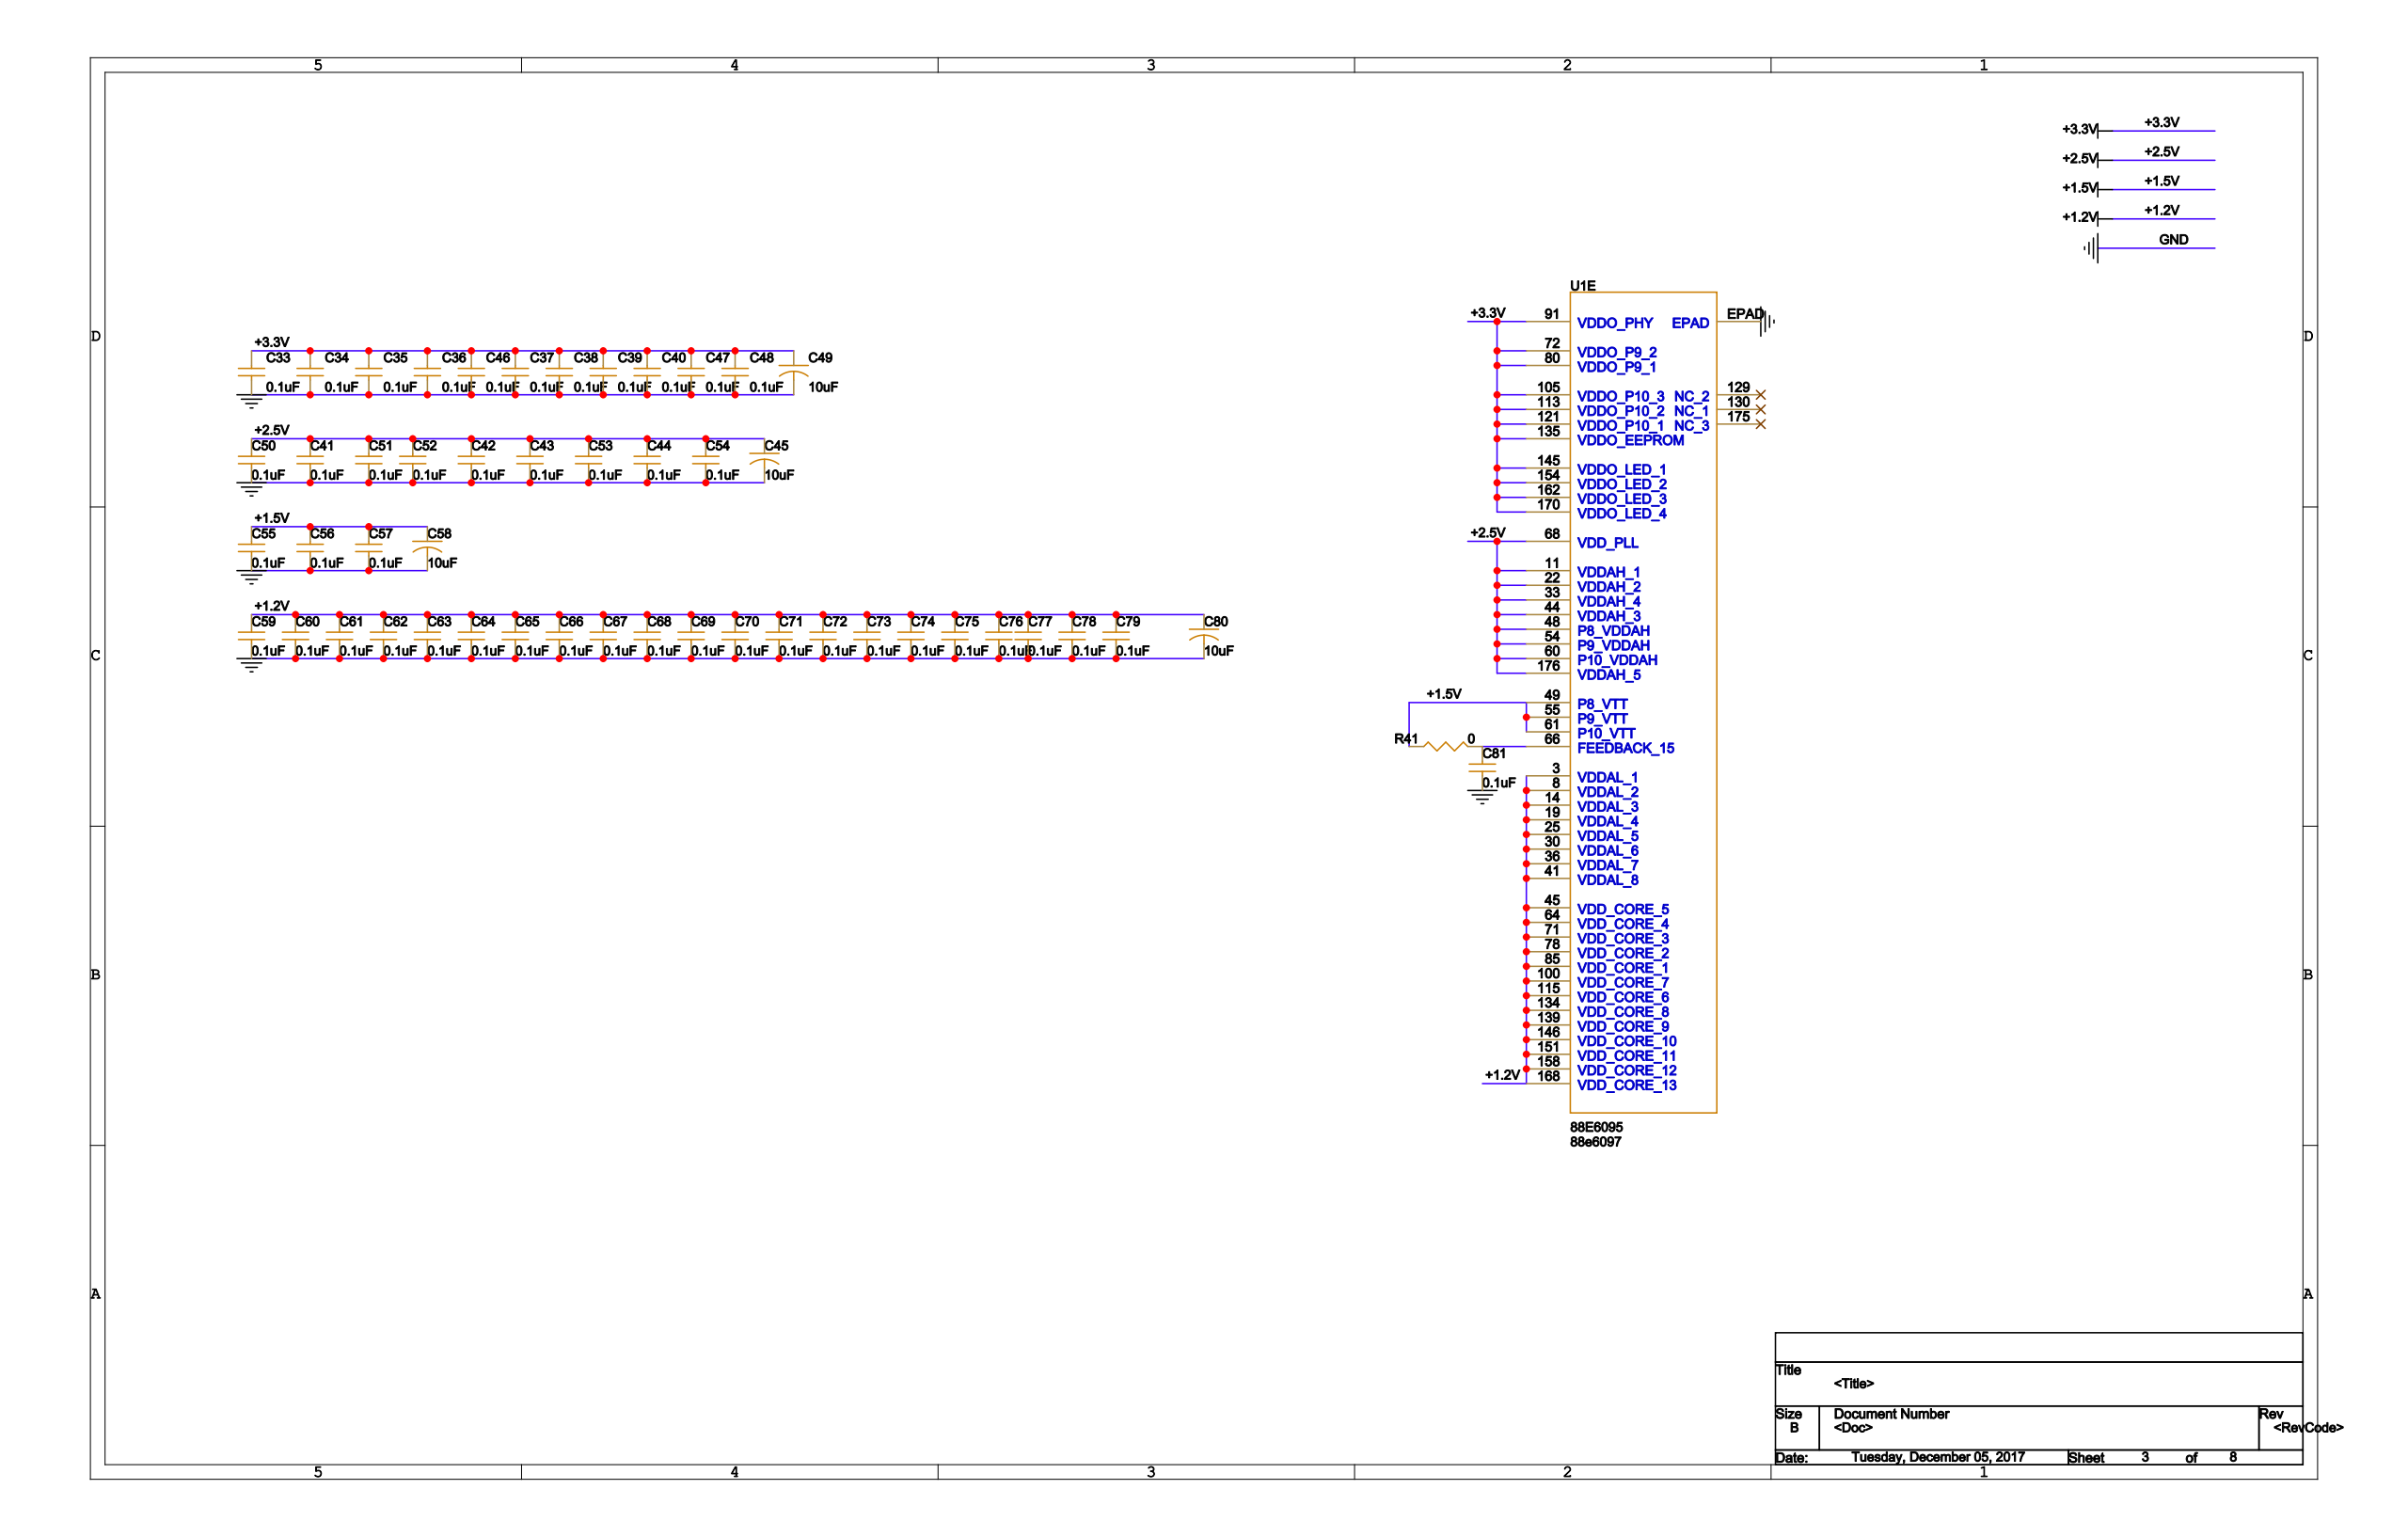Circuit board | Cadence Allegro | 219 parts | 174 nets | one sheet of the schematic
Parts on this sheet (reference | value | footprint):
C33 | 0.1uf | SC0603
C34 | 0.1uf | SC0603
C35 | 0.1uf | SC0603
C36 | 0.1uf | SC0603
C37 | 0.1uf | SC0603
C38 | 0.1uf | SC0603
C39 | 0.1uf | SC0603
C40 | 0.1uf | SC0603
C41 | 0.1uf | SC0603
C42 | 0.1uf | SC0603
C43 | 0.1uf | SC0603
C44 | 0.1uf | SC0603
C45 | 10uF | STC3528
C46 | 0.1uf | SC0603
C47 | 0.1uf | SC0603
C48 | 0.1uf | SC0603
C49 | 10uF | STC3528
C50 | 0.1uf | SC0603
C51 | 0.1uf | SC0603
C52 | 0.1uf | SC0603
C53 | 0.1uf | SC0603
C54 | 0.1uf | SC0603
C55 | 0.1uf | SC0603
C56 | 0.1uf | SC0603
C57 | 0.1uf | SC0603
C58 | 10uF | STC3528
C59 | 0.1uf | SC0603
C60 | 0.1uf | SC0603
C61 | 0.1uf | SC0603
C62 | 0.1uf | SC0603
C63 | 0.1uf | SC0603
C64 | 0.1uf | SC0603
C65 | 0.1uf | SC0603
C66 | 0.1uf | SC0603
C67 | 0.1uf | SC0603
C68 | 0.1uf | SC0603
C69 | 0.1uf | SC0603
C70 | 0.1uf | SC0603
C71 | 0.1uf | SC0603
C72 | 0.1uf | SC0603
C73 | 0.1uf | SC0603
C74 | 0.1uf | SC0603
C75 | 0.1uf | SC0603
C76 | 0.1uf | SC0603
C77 | 0.1uf | SC0603
C78 | 0.1uf | SC0603
C79 | 0.1uf | SC0603
C80 | 10uF | STC3528
C81 | 0.1uf | SC0603
R41 | 0 | SR0603
U1 | 88E6095 | 88E6097
Nets of these parts (net: part-pin ...):
GND: C33-2 C34-2 C35-2 C36-2 C37-2 C38-2 C39-2 C40-2 C41-2 C42-2 C43-2 C44-2 C45-2 C46-2 C47-2 C48-2 C49-2 C50-2 C51-2 C52-2 C53-2 C54-2 C55-2 C56-2 C57-2 C58-2 C59-2 C60-2 C61-2 C62-2 C63-2 C64-2 C65-2 C66-2 C67-2 C68-2 C69-2 C70-2 C71-2 C72-2 C73-2 C74-2 C75-2 C76-2 C77-2 C78-2 C79-2 C80-2 C81-2 U1-EPAD
N1336337: C81-1 R41-2 U1-66
+2.5V: C41-1 C42-1 C43-1 C44-1 C45-1 C50-1 C51-1 C52-1 C53-1 C54-1 U1-11 U1-22 U1-33 U1-44 U1-48 U1-54 U1-60 U1-68 U1-176
+1.5V: C55-1 C56-1 C57-1 C58-1 R41-1 U1-49 U1-55 U1-61
+1.2V: C59-1 C60-1 C61-1 C62-1 C63-1 C64-1 C65-1 C66-1 C67-1 C68-1 C69-1 C70-1 C71-1 C72-1 C73-1 C74-1 C75-1 C76-1 C77-1 C78-1 C79-1 C80-1 U1-3 U1-8 U1-14 U1-19 U1-25 U1-30 U1-36 U1-41 U1-45 U1-64 U1-71 U1-78 U1-85 U1-100 U1-115 U1-134 U1-139 U1-146 U1-151 U1-158 U1-168
+3.3V: C33-1 C34-1 C35-1 C36-1 C37-1 C38-1 C39-1 C40-1 C46-1 C47-1 C48-1 C49-1 U1-72 U1-80 U1-91 U1-105 U1-113 U1-121 U1-135 U1-145 U1-154 U1-162 U1-170